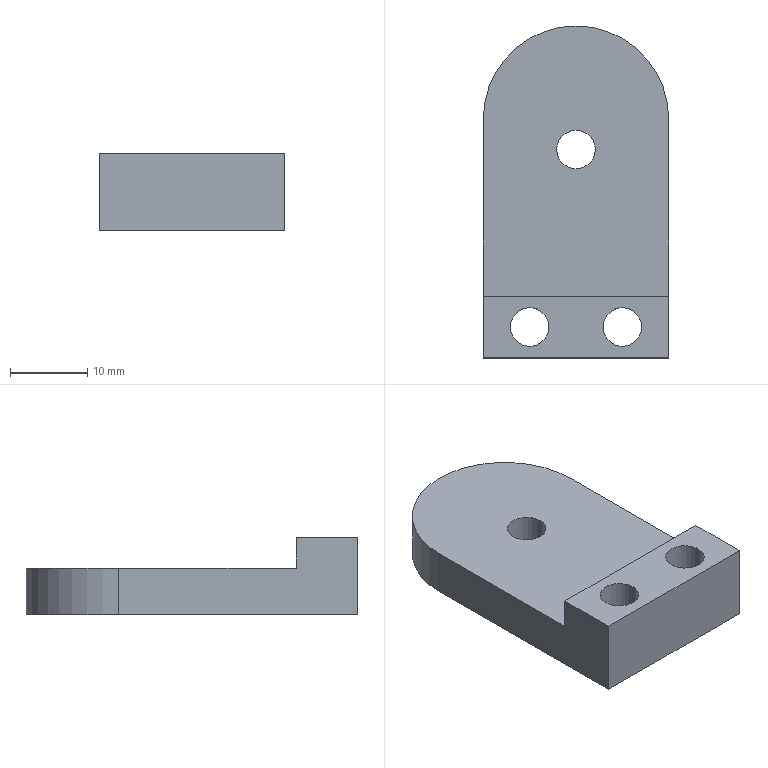Part | SolidWorks | features HoleWzd 2, Cut 1, Extrusion 1, Fillet 1 | 1 solid | 15 faces | box 24 x 43 x 10 mm | volume 6079 mm3 | cylinder 8 | plane 7 | commonest cylinder face diameters 5 x6 24 x2
STEP:
#1=CARTESIAN_POINT('',(20.5,4.,10.));
#2=VERTEX_POINT('',#1);
#3=CARTESIAN_POINT('',(15.5,4.,10.));
#4=VERTEX_POINT('',#3);
#5=CARTESIAN_POINT('',(18.,4.,10.));
#6=DIRECTION('',(0.,0.,-1.));
#7=DIRECTION('',(-1.,0.,0.));
#8=AXIS2_PLACEMENT_3D('',#5,#6,#7);
#9=CIRCLE('',#8,2.5);
#10=EDGE_CURVE('',#2,#4,#9,.T.);
#11=ORIENTED_EDGE('',*,*,#10,.F.);
#12=CARTESIAN_POINT('',(20.5,4.,0.));
#13=VERTEX_POINT('',#12);
#14=CARTESIAN_POINT('',(20.5,4.,0.));
#15=DIRECTION('',(0.,0.,-1.));
#16=VECTOR('',#15,1000.);
#17=LINE('',#14,#16);
#18=EDGE_CURVE('',#2,#13,#17,.T.);
#19=ORIENTED_EDGE('',*,*,#18,.T.);
#20=CARTESIAN_POINT('',(15.5,4.,0.));
#21=VERTEX_POINT('',#20);
#22=CARTESIAN_POINT('',(18.,4.,0.));
#23=DIRECTION('',(0.,0.,-1.));
#24=DIRECTION('',(-1.,0.,0.));
#25=AXIS2_PLACEMENT_3D('',#22,#23,#24);
#26=CIRCLE('',#25,2.5);
#27=EDGE_CURVE('',#13,#21,#26,.T.);
#28=ORIENTED_EDGE('',*,*,#27,.T.);
#29=CARTESIAN_POINT('',(15.5,4.,0.));
#30=DIRECTION('',(0.,0.,-1.));
#31=VECTOR('',#30,1000.);
#32=LINE('',#29,#31);
#33=EDGE_CURVE('',#4,#21,#32,.T.);
#34=ORIENTED_EDGE('',*,*,#33,.F.);
#35=EDGE_LOOP('',(#11,#19,#28,#34));
#36=FACE_OUTER_BOUND('',#35,.T.);
#37=CARTESIAN_POINT('',(18.,4.,0.));
#38=DIRECTION('',(0.,0.,-1.));
#39=DIRECTION('',(-1.,0.,0.));
#40=AXIS2_PLACEMENT_3D('',#37,#38,#39);
#41=CYLINDRICAL_SURFACE('',#40,2.5);
#42=ADVANCED_FACE('',(#36),#41,.F.);
#43=CARTESIAN_POINT('',(8.5,4.,10.));
#44=VERTEX_POINT('',#43);
#45=CARTESIAN_POINT('',(3.5,4.,10.));
#46=VERTEX_POINT('',#45);
#47=CARTESIAN_POINT('',(6.,4.,10.));
#48=DIRECTION('',(0.,0.,-1.));
#49=DIRECTION('',(-1.,0.,0.));
#50=AXIS2_PLACEMENT_3D('',#47,#48,#49);
#51=CIRCLE('',#50,2.5);
#52=EDGE_CURVE('',#44,#46,#51,.T.);
#53=ORIENTED_EDGE('',*,*,#52,.F.);
#54=CARTESIAN_POINT('',(8.5,4.,0.));
#55=VERTEX_POINT('',#54);
#56=CARTESIAN_POINT('',(8.5,4.,0.));
#57=DIRECTION('',(0.,0.,-1.));
#58=VECTOR('',#57,1000.);
#59=LINE('',#56,#58);
#60=EDGE_CURVE('',#44,#55,#59,.T.);
#61=ORIENTED_EDGE('',*,*,#60,.T.);
#62=CARTESIAN_POINT('',(3.5,4.,0.));
#63=VERTEX_POINT('',#62);
#64=CARTESIAN_POINT('',(6.,4.,0.));
#65=DIRECTION('',(0.,0.,-1.));
#66=DIRECTION('',(-1.,0.,0.));
#67=AXIS2_PLACEMENT_3D('',#64,#65,#66);
#68=CIRCLE('',#67,2.5);
#69=EDGE_CURVE('',#55,#63,#68,.T.);
#70=ORIENTED_EDGE('',*,*,#69,.T.);
#71=CARTESIAN_POINT('',(3.5,4.,0.));
#72=DIRECTION('',(0.,0.,-1.));
#73=VECTOR('',#72,1000.);
#74=LINE('',#71,#73);
#75=EDGE_CURVE('',#46,#63,#74,.T.);
#76=ORIENTED_EDGE('',*,*,#75,.F.);
#77=EDGE_LOOP('',(#53,#61,#70,#76));
#78=FACE_OUTER_BOUND('',#77,.T.);
#79=CARTESIAN_POINT('',(6.,4.,0.));
#80=DIRECTION('',(0.,0.,-1.));
#81=DIRECTION('',(-1.,0.,0.));
#82=AXIS2_PLACEMENT_3D('',#79,#80,#81);
#83=CYLINDRICAL_SURFACE('',#82,2.5);
#84=ADVANCED_FACE('',(#78),#83,.F.);
#85=CARTESIAN_POINT('',(14.5,27.,6.));
#86=VERTEX_POINT('',#85);
#87=CARTESIAN_POINT('',(9.5,27.,6.));
#88=VERTEX_POINT('',#87);
#89=CARTESIAN_POINT('',(12.,27.,6.));
#90=DIRECTION('',(0.,0.,-1.));
#91=DIRECTION('',(0.,1.,0.));
#92=AXIS2_PLACEMENT_3D('',#89,#90,#91);
#93=CIRCLE('',#92,2.5);
#94=EDGE_CURVE('',#86,#88,#93,.T.);
#95=ORIENTED_EDGE('',*,*,#94,.F.);
#96=CARTESIAN_POINT('',(14.5,27.,0.));
#97=VERTEX_POINT('',#96);
#98=CARTESIAN_POINT('',(14.5,27.,0.));
#99=DIRECTION('',(0.,0.,-1.));
#100=VECTOR('',#99,1000.);
#101=LINE('',#98,#100);
#102=EDGE_CURVE('',#86,#97,#101,.T.);
#103=ORIENTED_EDGE('',*,*,#102,.T.);
#104=CARTESIAN_POINT('',(9.5,27.,0.));
#105=VERTEX_POINT('',#104);
#106=CARTESIAN_POINT('',(12.,27.,0.));
#107=DIRECTION('',(0.,0.,-1.));
#108=DIRECTION('',(-1.,0.,0.));
#109=AXIS2_PLACEMENT_3D('',#106,#107,#108);
#110=CIRCLE('',#109,2.5);
#111=EDGE_CURVE('',#97,#105,#110,.T.);
#112=ORIENTED_EDGE('',*,*,#111,.T.);
#113=CARTESIAN_POINT('',(9.5,27.,0.));
#114=DIRECTION('',(0.,0.,-1.));
#115=VECTOR('',#114,1000.);
#116=LINE('',#113,#115);
#117=EDGE_CURVE('',#88,#105,#116,.T.);
#118=ORIENTED_EDGE('',*,*,#117,.F.);
#119=EDGE_LOOP('',(#95,#103,#112,#118));
#120=FACE_OUTER_BOUND('',#119,.T.);
#121=CARTESIAN_POINT('',(12.,27.,0.));
#122=DIRECTION('',(0.,0.,-1.));
#123=DIRECTION('',(-1.,0.,0.));
#124=AXIS2_PLACEMENT_3D('',#121,#122,#123);
#125=CYLINDRICAL_SURFACE('',#124,2.5);
#126=ADVANCED_FACE('',(#120),#125,.F.);
#127=CARTESIAN_POINT('',(0.,8.,6.));
#128=VERTEX_POINT('',#127);
#129=CARTESIAN_POINT('',(0.,31.,6.));
#130=VERTEX_POINT('',#129);
#131=CARTESIAN_POINT('',(0.,0.,6.));
#132=DIRECTION('',(0.,1.,0.));
#133=VECTOR('',#132,1000.);
#134=LINE('',#131,#133);
#135=EDGE_CURVE('',#128,#130,#134,.T.);
#136=ORIENTED_EDGE('',*,*,#135,.T.);
#137=CARTESIAN_POINT('',(0.,31.,0.));
#138=VERTEX_POINT('',#137);
#139=CARTESIAN_POINT('',(0.,31.,10.));
#140=DIRECTION('',(0.,0.,-1.));
#141=VECTOR('',#140,1000.);
#142=LINE('',#139,#141);
#143=EDGE_CURVE('',#130,#138,#142,.T.);
#144=ORIENTED_EDGE('',*,*,#143,.T.);
#145=CARTESIAN_POINT('',(0.,0.,0.));
#146=VERTEX_POINT('',#145);
#147=CARTESIAN_POINT('',(0.,0.,0.));
#148=DIRECTION('',(0.,-1.,0.));
#149=VECTOR('',#148,1000.);
#150=LINE('',#147,#149);
#151=EDGE_CURVE('',#138,#146,#150,.T.);
#152=ORIENTED_EDGE('',*,*,#151,.T.);
#153=CARTESIAN_POINT('',(0.,0.,10.));
#154=VERTEX_POINT('',#153);
#155=CARTESIAN_POINT('',(0.,0.,10.));
#156=DIRECTION('',(0.,0.,-1.));
#157=VECTOR('',#156,1000.);
#158=LINE('',#155,#157);
#159=EDGE_CURVE('',#154,#146,#158,.T.);
#160=ORIENTED_EDGE('',*,*,#159,.F.);
#161=CARTESIAN_POINT('',(0.,8.,10.));
#162=VERTEX_POINT('',#161);
#163=CARTESIAN_POINT('',(0.,0.,10.));
#164=DIRECTION('',(0.,-1.,0.));
#165=VECTOR('',#164,1000.);
#166=LINE('',#163,#165);
#167=EDGE_CURVE('',#162,#154,#166,.T.);
#168=ORIENTED_EDGE('',*,*,#167,.F.);
#169=CARTESIAN_POINT('',(0.,8.,10.));
#170=DIRECTION('',(0.,0.,-1.));
#171=VECTOR('',#170,1000.);
#172=LINE('',#169,#171);
#173=EDGE_CURVE('',#162,#128,#172,.T.);
#174=ORIENTED_EDGE('',*,*,#173,.T.);
#175=EDGE_LOOP('',(#136,#144,#152,#160,#168,#174));
#176=FACE_OUTER_BOUND('',#175,.T.);
#177=CARTESIAN_POINT('',(0.,0.,10.));
#178=DIRECTION('',(1.,0.,0.));
#179=DIRECTION('',(0.,0.,-1.));
#180=AXIS2_PLACEMENT_3D('',#177,#178,#179);
#181=PLANE('',#180);
#182=ADVANCED_FACE('',(#176),#181,.F.);
#183=CARTESIAN_POINT('',(24.,0.,0.));
#184=VERTEX_POINT('',#183);
#185=CARTESIAN_POINT('',(0.,0.,0.));
#186=DIRECTION('',(1.,0.,0.));
#187=VECTOR('',#186,1000.);
#188=LINE('',#185,#187);
#189=EDGE_CURVE('',#146,#184,#188,.T.);
#190=ORIENTED_EDGE('',*,*,#189,.T.);
#191=CARTESIAN_POINT('',(24.,0.,10.));
#192=VERTEX_POINT('',#191);
#193=CARTESIAN_POINT('',(24.,0.,10.));
#194=DIRECTION('',(0.,0.,-1.));
#195=VECTOR('',#194,1000.);
#196=LINE('',#193,#195);
#197=EDGE_CURVE('',#192,#184,#196,.T.);
#198=ORIENTED_EDGE('',*,*,#197,.F.);
#199=CARTESIAN_POINT('',(0.,0.,10.));
#200=DIRECTION('',(1.,0.,0.));
#201=VECTOR('',#200,1000.);
#202=LINE('',#199,#201);
#203=EDGE_CURVE('',#154,#192,#202,.T.);
#204=ORIENTED_EDGE('',*,*,#203,.F.);
#205=ORIENTED_EDGE('',*,*,#159,.T.);
#206=EDGE_LOOP('',(#190,#198,#204,#205));
#207=FACE_OUTER_BOUND('',#206,.T.);
#208=CARTESIAN_POINT('',(0.,0.,10.));
#209=DIRECTION('',(0.,1.,0.));
#210=DIRECTION('',(0.,0.,1.));
#211=AXIS2_PLACEMENT_3D('',#208,#209,#210);
#212=PLANE('',#211);
#213=ADVANCED_FACE('',(#207),#212,.F.);
#214=CARTESIAN_POINT('',(24.,31.,0.));
#215=VERTEX_POINT('',#214);
#216=CARTESIAN_POINT('',(24.,0.,0.));
#217=DIRECTION('',(0.,1.,0.));
#218=VECTOR('',#217,1000.);
#219=LINE('',#216,#218);
#220=EDGE_CURVE('',#184,#215,#219,.T.);
#221=ORIENTED_EDGE('',*,*,#220,.T.);
#222=CARTESIAN_POINT('',(24.,31.,6.));
#223=VERTEX_POINT('',#222);
#224=CARTESIAN_POINT('',(24.,31.,10.));
#225=DIRECTION('',(0.,0.,1.));
#226=VECTOR('',#225,1000.);
#227=LINE('',#224,#226);
#228=EDGE_CURVE('',#215,#223,#227,.T.);
#229=ORIENTED_EDGE('',*,*,#228,.T.);
#230=CARTESIAN_POINT('',(24.,8.,6.));
#231=VERTEX_POINT('',#230);
#232=CARTESIAN_POINT('',(24.,43.,6.));
#233=DIRECTION('',(0.,1.,0.));
#234=VECTOR('',#233,1000.);
#235=LINE('',#232,#234);
#236=EDGE_CURVE('',#231,#223,#235,.T.);
#237=ORIENTED_EDGE('',*,*,#236,.F.);
#238=CARTESIAN_POINT('',(24.,8.,10.));
#239=VERTEX_POINT('',#238);
#240=CARTESIAN_POINT('',(24.,8.,10.));
#241=DIRECTION('',(0.,0.,-1.));
#242=VECTOR('',#241,1000.);
#243=LINE('',#240,#242);
#244=EDGE_CURVE('',#239,#231,#243,.T.);
#245=ORIENTED_EDGE('',*,*,#244,.F.);
#246=CARTESIAN_POINT('',(24.,0.,10.));
#247=DIRECTION('',(0.,1.,0.));
#248=VECTOR('',#247,1000.);
#249=LINE('',#246,#248);
#250=EDGE_CURVE('',#192,#239,#249,.T.);
#251=ORIENTED_EDGE('',*,*,#250,.F.);
#252=ORIENTED_EDGE('',*,*,#197,.T.);
#253=EDGE_LOOP('',(#221,#229,#237,#245,#251,#252));
#254=FACE_OUTER_BOUND('',#253,.T.);
#255=CARTESIAN_POINT('',(24.,0.,10.));
#256=DIRECTION('',(-1.,0.,0.));
#257=DIRECTION('',(0.,0.,1.));
#258=AXIS2_PLACEMENT_3D('',#255,#256,#257);
#259=PLANE('',#258);
#260=ADVANCED_FACE('',(#254),#259,.F.);
#261=CARTESIAN_POINT('',(18.,4.,10.));
#262=DIRECTION('',(0.,0.,-1.));
#263=DIRECTION('',(-1.,0.,0.));
#264=AXIS2_PLACEMENT_3D('',#261,#262,#263);
#265=CIRCLE('',#264,2.5);
#266=EDGE_CURVE('',#4,#2,#265,.T.);
#267=ORIENTED_EDGE('',*,*,#266,.T.);
#268=ORIENTED_EDGE('',*,*,#10,.T.);
#269=EDGE_LOOP('',(#267,#268));
#270=FACE_BOUND('',#269,.T.);
#271=CARTESIAN_POINT('',(6.,4.,10.));
#272=DIRECTION('',(0.,0.,-1.));
#273=DIRECTION('',(-1.,0.,0.));
#274=AXIS2_PLACEMENT_3D('',#271,#272,#273);
#275=CIRCLE('',#274,2.5);
#276=EDGE_CURVE('',#46,#44,#275,.T.);
#277=ORIENTED_EDGE('',*,*,#276,.T.);
#278=ORIENTED_EDGE('',*,*,#52,.T.);
#279=EDGE_LOOP('',(#277,#278));
#280=FACE_BOUND('',#279,.T.);
#281=ORIENTED_EDGE('',*,*,#250,.T.);
#282=CARTESIAN_POINT('',(0.,8.,10.));
#283=DIRECTION('',(-1.,0.,0.));
#284=VECTOR('',#283,1000.);
#285=LINE('',#282,#284);
#286=EDGE_CURVE('',#239,#162,#285,.T.);
#287=ORIENTED_EDGE('',*,*,#286,.T.);
#288=ORIENTED_EDGE('',*,*,#167,.T.);
#289=ORIENTED_EDGE('',*,*,#203,.T.);
#290=EDGE_LOOP('',(#281,#287,#288,#289));
#291=FACE_OUTER_BOUND('',#290,.T.);
#292=CARTESIAN_POINT('',(0.,0.,10.));
#293=DIRECTION('',(0.,0.,-1.));
#294=DIRECTION('',(-1.,0.,0.));
#295=AXIS2_PLACEMENT_3D('',#292,#293,#294);
#296=PLANE('',#295);
#297=ADVANCED_FACE('',(#270,#280,#291),#296,.F.);
#298=CARTESIAN_POINT('',(18.,4.,0.));
#299=DIRECTION('',(0.,0.,-1.));
#300=DIRECTION('',(-1.,0.,0.));
#301=AXIS2_PLACEMENT_3D('',#298,#299,#300);
#302=CIRCLE('',#301,2.5);
#303=EDGE_CURVE('',#21,#13,#302,.T.);
#304=ORIENTED_EDGE('',*,*,#303,.F.);
#305=ORIENTED_EDGE('',*,*,#27,.F.);
#306=EDGE_LOOP('',(#304,#305));
#307=FACE_BOUND('',#306,.T.);
#308=CARTESIAN_POINT('',(6.,4.,0.));
#309=DIRECTION('',(0.,0.,-1.));
#310=DIRECTION('',(-1.,0.,0.));
#311=AXIS2_PLACEMENT_3D('',#308,#309,#310);
#312=CIRCLE('',#311,2.5);
#313=EDGE_CURVE('',#63,#55,#312,.T.);
#314=ORIENTED_EDGE('',*,*,#313,.F.);
#315=ORIENTED_EDGE('',*,*,#69,.F.);
#316=EDGE_LOOP('',(#314,#315));
#317=FACE_BOUND('',#316,.T.);
#318=CARTESIAN_POINT('',(12.,27.,0.));
#319=DIRECTION('',(0.,0.,-1.));
#320=DIRECTION('',(-1.,0.,0.));
#321=AXIS2_PLACEMENT_3D('',#318,#319,#320);
#322=CIRCLE('',#321,2.5);
#323=EDGE_CURVE('',#105,#97,#322,.T.);
#324=ORIENTED_EDGE('',*,*,#323,.F.);
#325=ORIENTED_EDGE('',*,*,#111,.F.);
#326=EDGE_LOOP('',(#324,#325));
#327=FACE_BOUND('',#326,.T.);
#328=ORIENTED_EDGE('',*,*,#151,.F.);
#329=CARTESIAN_POINT('',(12.,43.,0.));
#330=VERTEX_POINT('',#329);
#331=CARTESIAN_POINT('',(12.,31.,0.));
#332=DIRECTION('',(0.,0.,-1.));
#333=DIRECTION('',(-1.,0.,0.));
#334=AXIS2_PLACEMENT_3D('',#331,#332,#333);
#335=CIRCLE('',#334,12.);
#336=EDGE_CURVE('',#138,#330,#335,.T.);
#337=ORIENTED_EDGE('',*,*,#336,.T.);
#338=CARTESIAN_POINT('',(12.,31.,0.));
#339=DIRECTION('',(0.,0.,-1.));
#340=DIRECTION('',(-1.,0.,0.));
#341=AXIS2_PLACEMENT_3D('',#338,#339,#340);
#342=CIRCLE('',#341,12.);
#343=EDGE_CURVE('',#330,#215,#342,.T.);
#344=ORIENTED_EDGE('',*,*,#343,.T.);
#345=ORIENTED_EDGE('',*,*,#220,.F.);
#346=ORIENTED_EDGE('',*,*,#189,.F.);
#347=EDGE_LOOP('',(#328,#337,#344,#345,#346));
#348=FACE_OUTER_BOUND('',#347,.T.);
#349=CARTESIAN_POINT('',(0.,0.,0.));
#350=DIRECTION('',(0.,0.,-1.));
#351=DIRECTION('',(-1.,0.,0.));
#352=AXIS2_PLACEMENT_3D('',#349,#350,#351);
#353=PLANE('',#352);
#354=ADVANCED_FACE('',(#307,#317,#327,#348),#353,.T.);
#355=CARTESIAN_POINT('',(12.,27.,6.));
#356=DIRECTION('',(0.,0.,-1.));
#357=DIRECTION('',(0.,1.,0.));
#358=AXIS2_PLACEMENT_3D('',#355,#356,#357);
#359=CIRCLE('',#358,2.5);
#360=EDGE_CURVE('',#88,#86,#359,.T.);
#361=ORIENTED_EDGE('',*,*,#360,.T.);
#362=ORIENTED_EDGE('',*,*,#94,.T.);
#363=EDGE_LOOP('',(#361,#362));
#364=FACE_BOUND('',#363,.T.);
#365=CARTESIAN_POINT('',(12.,43.,6.));
#366=VERTEX_POINT('',#365);
#367=CARTESIAN_POINT('',(12.,31.,6.));
#368=DIRECTION('',(0.,0.,1.));
#369=DIRECTION('',(0.,1.,0.));
#370=AXIS2_PLACEMENT_3D('',#367,#368,#369);
#371=CIRCLE('',#370,12.);
#372=EDGE_CURVE('',#223,#366,#371,.T.);
#373=ORIENTED_EDGE('',*,*,#372,.T.);
#374=CARTESIAN_POINT('',(12.,31.,6.));
#375=DIRECTION('',(0.,0.,1.));
#376=DIRECTION('',(0.,1.,0.));
#377=AXIS2_PLACEMENT_3D('',#374,#375,#376);
#378=CIRCLE('',#377,12.);
#379=EDGE_CURVE('',#366,#130,#378,.T.);
#380=ORIENTED_EDGE('',*,*,#379,.T.);
#381=ORIENTED_EDGE('',*,*,#135,.F.);
#382=CARTESIAN_POINT('',(-18.,8.,6.));
#383=DIRECTION('',(1.,0.,0.));
#384=VECTOR('',#383,1000.);
#385=LINE('',#382,#384);
#386=EDGE_CURVE('',#128,#231,#385,.T.);
#387=ORIENTED_EDGE('',*,*,#386,.T.);
#388=ORIENTED_EDGE('',*,*,#236,.T.);
#389=EDGE_LOOP('',(#373,#380,#381,#387,#388));
#390=FACE_OUTER_BOUND('',#389,.T.);
#391=CARTESIAN_POINT('',(-18.,43.,6.));
#392=DIRECTION('',(0.,0.,-1.));
#393=DIRECTION('',(0.,1.,0.));
#394=AXIS2_PLACEMENT_3D('',#391,#392,#393);
#395=PLANE('',#394);
#396=ADVANCED_FACE('',(#364,#390),#395,.F.);
#397=ORIENTED_EDGE('',*,*,#286,.F.);
#398=ORIENTED_EDGE('',*,*,#244,.T.);
#399=ORIENTED_EDGE('',*,*,#386,.F.);
#400=ORIENTED_EDGE('',*,*,#173,.F.);
#401=EDGE_LOOP('',(#397,#398,#399,#400));
#402=FACE_OUTER_BOUND('',#401,.T.);
#403=CARTESIAN_POINT('',(-18.,8.,10.));
#404=DIRECTION('',(0.,-1.,0.));
#405=DIRECTION('',(0.,0.,-1.));
#406=AXIS2_PLACEMENT_3D('',#403,#404,#405);
#407=PLANE('',#406);
#408=ADVANCED_FACE('',(#402),#407,.F.);
#409=ORIENTED_EDGE('',*,*,#102,.F.);
#410=ORIENTED_EDGE('',*,*,#360,.F.);
#411=ORIENTED_EDGE('',*,*,#117,.T.);
#412=ORIENTED_EDGE('',*,*,#323,.T.);
#413=EDGE_LOOP('',(#409,#410,#411,#412));
#414=FACE_OUTER_BOUND('',#413,.T.);
#415=CARTESIAN_POINT('',(12.,27.,0.));
#416=DIRECTION('',(0.,0.,-1.));
#417=DIRECTION('',(-1.,0.,0.));
#418=AXIS2_PLACEMENT_3D('',#415,#416,#417);
#419=CYLINDRICAL_SURFACE('',#418,2.5);
#420=ADVANCED_FACE('',(#414),#419,.F.);
#421=CARTESIAN_POINT('',(12.,43.,10.));
#422=DIRECTION('',(0.,0.,-1.));
#423=VECTOR('',#422,1000.);
#424=LINE('',#421,#423);
#425=EDGE_CURVE('',#366,#330,#424,.T.);
#426=ORIENTED_EDGE('',*,*,#425,.F.);
#427=ORIENTED_EDGE('',*,*,#372,.F.);
#428=ORIENTED_EDGE('',*,*,#228,.F.);
#429=ORIENTED_EDGE('',*,*,#343,.F.);
#430=EDGE_LOOP('',(#426,#427,#428,#429));
#431=FACE_OUTER_BOUND('',#430,.T.);
#432=CARTESIAN_POINT('',(12.,31.,10.));
#433=DIRECTION('',(0.,0.,-1.));
#434=DIRECTION('',(-1.,0.,0.));
#435=AXIS2_PLACEMENT_3D('',#432,#433,#434);
#436=CYLINDRICAL_SURFACE('',#435,12.);
#437=ADVANCED_FACE('',(#431),#436,.T.);
#438=ORIENTED_EDGE('',*,*,#379,.F.);
#439=ORIENTED_EDGE('',*,*,#425,.T.);
#440=ORIENTED_EDGE('',*,*,#336,.F.);
#441=ORIENTED_EDGE('',*,*,#143,.F.);
#442=EDGE_LOOP('',(#438,#439,#440,#441));
#443=FACE_OUTER_BOUND('',#442,.T.);
#444=CARTESIAN_POINT('',(12.,31.,10.));
#445=DIRECTION('',(0.,0.,-1.));
#446=DIRECTION('',(-1.,0.,0.));
#447=AXIS2_PLACEMENT_3D('',#444,#445,#446);
#448=CYLINDRICAL_SURFACE('',#447,12.);
#449=ADVANCED_FACE('',(#443),#448,.T.);
#450=ORIENTED_EDGE('',*,*,#60,.F.);
#451=ORIENTED_EDGE('',*,*,#276,.F.);
#452=ORIENTED_EDGE('',*,*,#75,.T.);
#453=ORIENTED_EDGE('',*,*,#313,.T.);
#454=EDGE_LOOP('',(#450,#451,#452,#453));
#455=FACE_OUTER_BOUND('',#454,.T.);
#456=CARTESIAN_POINT('',(6.,4.,0.));
#457=DIRECTION('',(0.,0.,-1.));
#458=DIRECTION('',(-1.,0.,0.));
#459=AXIS2_PLACEMENT_3D('',#456,#457,#458);
#460=CYLINDRICAL_SURFACE('',#459,2.5);
#461=ADVANCED_FACE('',(#455),#460,.F.);
#462=ORIENTED_EDGE('',*,*,#18,.F.);
#463=ORIENTED_EDGE('',*,*,#266,.F.);
#464=ORIENTED_EDGE('',*,*,#33,.T.);
#465=ORIENTED_EDGE('',*,*,#303,.T.);
#466=EDGE_LOOP('',(#462,#463,#464,#465));
#467=FACE_OUTER_BOUND('',#466,.T.);
#468=CARTESIAN_POINT('',(18.,4.,0.));
#469=DIRECTION('',(0.,0.,-1.));
#470=DIRECTION('',(-1.,0.,0.));
#471=AXIS2_PLACEMENT_3D('',#468,#469,#470);
#472=CYLINDRICAL_SURFACE('',#471,2.5);
#473=ADVANCED_FACE('',(#467),#472,.F.);
#474=CLOSED_SHELL('',(#42,#84,#126,#182,#213,#260,#297,#354,#396,#408,#420,#437,#449,#461,#473));
#475=MANIFOLD_SOLID_BREP('',#474);
#476=CARTESIAN_POINT('',(0.,0.,0.));
#477=DIRECTION('',(0.,0.,1.));
#478=DIRECTION('',(1.,0.,0.));
#479=AXIS2_PLACEMENT_3D('',#476,#477,#478);
#480=(LENGTH_UNIT()NAMED_UNIT(*)SI_UNIT(.MILLI.,.METRE.));
#481=UNCERTAINTY_MEASURE_WITH_UNIT(LENGTH_MEASURE(0.00001),#480,'','');
#482=(NAMED_UNIT(*)PLANE_ANGLE_UNIT()SI_UNIT($,.RADIAN.));
#483=(NAMED_UNIT(*)SI_UNIT($,.STERADIAN.)SOLID_ANGLE_UNIT());
#484=(GEOMETRIC_REPRESENTATION_CONTEXT(3)GLOBAL_UNCERTAINTY_ASSIGNED_CONTEXT((#481))GLOBAL_UNIT_ASSIGNED_CONTEXT((#480,#482,#483))REPRESENTATION_CONTEXT('',''));
#485=ADVANCED_BREP_SHAPE_REPRESENTATION('',(#475,#479),#484);